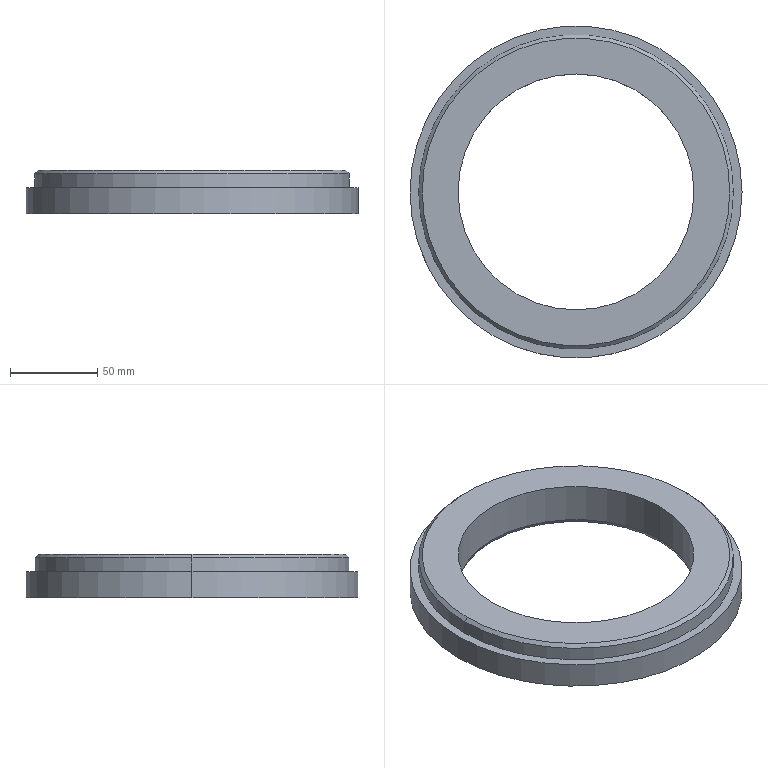Part | SolidWorks | features Chamfer 2, 3DProfileFeature 1, Extrusion 1, HoleWzd 1, ICE 1 | 1 solid | 37 faces | box 190 x 190 x 25 mm | volume 309604 mm3 | cylinder 18 | cone 16 | plane 3 | commonest cylinder face diameters 10.5 x12 135 x2 180 x2 190 x2
STEP:
#1=CARTESIAN_POINT('',(45.5,69.715,20.));
#2=VERTEX_POINT('',#1);
#3=CARTESIAN_POINT('',(35.,69.715,20.));
#4=VERTEX_POINT('',#3);
#5=CARTESIAN_POINT('',(40.25,69.715,20.));
#6=DIRECTION('',(0.,0.,-1.));
#7=DIRECTION('',(-1.,0.,0.));
#8=AXIS2_PLACEMENT_3D('',#5,#6,#7);
#9=CIRCLE('',#8,5.25);
#10=EDGE_CURVE('',#2,#4,#9,.T.);
#11=ORIENTED_EDGE('',*,*,#10,.F.);
#12=CARTESIAN_POINT('',(45.5,69.715,0.));
#13=VERTEX_POINT('',#12);
#14=CARTESIAN_POINT('',(45.5,69.715,0.));
#15=DIRECTION('',(0.,0.,-1.));
#16=VECTOR('',#15,1000.);
#17=LINE('',#14,#16);
#18=EDGE_CURVE('',#2,#13,#17,.T.);
#19=ORIENTED_EDGE('',*,*,#18,.T.);
#20=CARTESIAN_POINT('',(35.,69.715,0.));
#21=VERTEX_POINT('',#20);
#22=CARTESIAN_POINT('',(40.25,69.715,0.));
#23=DIRECTION('',(0.,0.,-1.));
#24=DIRECTION('',(-1.,0.,0.));
#25=AXIS2_PLACEMENT_3D('',#22,#23,#24);
#26=CIRCLE('',#25,5.25);
#27=EDGE_CURVE('',#13,#21,#26,.T.);
#28=ORIENTED_EDGE('',*,*,#27,.T.);
#29=CARTESIAN_POINT('',(35.,69.715,0.));
#30=DIRECTION('',(0.,0.,-1.));
#31=VECTOR('',#30,1000.);
#32=LINE('',#29,#31);
#33=EDGE_CURVE('',#4,#21,#32,.T.);
#34=ORIENTED_EDGE('',*,*,#33,.F.);
#35=EDGE_LOOP('',(#11,#19,#28,#34));
#36=FACE_OUTER_BOUND('',#35,.T.);
#37=CARTESIAN_POINT('',(40.25,69.715,0.));
#38=DIRECTION('',(0.,0.,-1.));
#39=DIRECTION('',(-1.,0.,0.));
#40=AXIS2_PLACEMENT_3D('',#37,#38,#39);
#41=CYLINDRICAL_SURFACE('',#40,5.25);
#42=ADVANCED_FACE('',(#36),#41,.F.);
#43=CARTESIAN_POINT('',(40.25,69.715,23.155));
#44=VERTEX_POINT('',#43);
#45=CARTESIAN_POINT('',(35.,69.715,20.));
#46=DIRECTION('',(-0.8572,0.,-0.515));
#47=VECTOR('',#46,1000.);
#48=LINE('',#45,#47);
#49=EDGE_CURVE('',#44,#4,#48,.T.);
#50=ORIENTED_EDGE('',*,*,#49,.F.);
#51=CARTESIAN_POINT('',(45.5,69.715,20.));
#52=DIRECTION('',(0.8572,0.,-0.515));
#53=VECTOR('',#52,1000.);
#54=LINE('',#51,#53);
#55=EDGE_CURVE('',#44,#2,#54,.T.);
#56=ORIENTED_EDGE('',*,*,#55,.T.);
#57=ORIENTED_EDGE('',*,*,#10,.T.);
#58=EDGE_LOOP('',(#50,#56,#57));
#59=FACE_OUTER_BOUND('',#58,.T.);
#60=CARTESIAN_POINT('',(40.25,69.715,20.));
#61=DIRECTION('',(0.,0.,-1.));
#62=DIRECTION('',(-1.,0.,0.));
#63=AXIS2_PLACEMENT_3D('',#60,#61,#62);
#64=CONICAL_SURFACE('',#63,5.25,1.03);
#65=ADVANCED_FACE('',(#59),#64,.F.);
#66=CARTESIAN_POINT('',(-35.,69.715,20.));
#67=VERTEX_POINT('',#66);
#68=CARTESIAN_POINT('',(-45.5,69.715,20.));
#69=VERTEX_POINT('',#68);
#70=CARTESIAN_POINT('',(-40.25,69.715,20.));
#71=DIRECTION('',(0.,0.,-1.));
#72=DIRECTION('',(-1.,0.,0.));
#73=AXIS2_PLACEMENT_3D('',#70,#71,#72);
#74=CIRCLE('',#73,5.25);
#75=EDGE_CURVE('',#67,#69,#74,.T.);
#76=ORIENTED_EDGE('',*,*,#75,.F.);
#77=CARTESIAN_POINT('',(-35.,69.715,0.));
#78=VERTEX_POINT('',#77);
#79=CARTESIAN_POINT('',(-35.,69.715,0.));
#80=DIRECTION('',(0.,0.,-1.));
#81=VECTOR('',#80,1000.);
#82=LINE('',#79,#81);
#83=EDGE_CURVE('',#67,#78,#82,.T.);
#84=ORIENTED_EDGE('',*,*,#83,.T.);
#85=CARTESIAN_POINT('',(-45.5,69.715,0.));
#86=VERTEX_POINT('',#85);
#87=CARTESIAN_POINT('',(-40.25,69.715,0.));
#88=DIRECTION('',(0.,0.,-1.));
#89=DIRECTION('',(-1.,0.,0.));
#90=AXIS2_PLACEMENT_3D('',#87,#88,#89);
#91=CIRCLE('',#90,5.25);
#92=EDGE_CURVE('',#78,#86,#91,.T.);
#93=ORIENTED_EDGE('',*,*,#92,.T.);
#94=CARTESIAN_POINT('',(-45.5,69.715,0.));
#95=DIRECTION('',(0.,0.,-1.));
#96=VECTOR('',#95,1000.);
#97=LINE('',#94,#96);
#98=EDGE_CURVE('',#69,#86,#97,.T.);
#99=ORIENTED_EDGE('',*,*,#98,.F.);
#100=EDGE_LOOP('',(#76,#84,#93,#99));
#101=FACE_OUTER_BOUND('',#100,.T.);
#102=CARTESIAN_POINT('',(-40.25,69.715,0.));
#103=DIRECTION('',(0.,0.,-1.));
#104=DIRECTION('',(-1.,0.,0.));
#105=AXIS2_PLACEMENT_3D('',#102,#103,#104);
#106=CYLINDRICAL_SURFACE('',#105,5.25);
#107=ADVANCED_FACE('',(#101),#106,.F.);
#108=CARTESIAN_POINT('',(-40.25,69.715,23.155));
#109=VERTEX_POINT('',#108);
#110=CARTESIAN_POINT('',(-45.5,69.715,20.));
#111=DIRECTION('',(-0.8572,0.,-0.515));
#112=VECTOR('',#111,1000.);
#113=LINE('',#110,#112);
#114=EDGE_CURVE('',#109,#69,#113,.T.);
#115=ORIENTED_EDGE('',*,*,#114,.F.);
#116=CARTESIAN_POINT('',(-35.,69.715,20.));
#117=DIRECTION('',(0.8572,0.,-0.515));
#118=VECTOR('',#117,1000.);
#119=LINE('',#116,#118);
#120=EDGE_CURVE('',#109,#67,#119,.T.);
#121=ORIENTED_EDGE('',*,*,#120,.T.);
#122=ORIENTED_EDGE('',*,*,#75,.T.);
#123=EDGE_LOOP('',(#115,#121,#122));
#124=FACE_OUTER_BOUND('',#123,.T.);
#125=CARTESIAN_POINT('',(-40.25,69.715,20.));
#126=DIRECTION('',(0.,0.,-1.));
#127=DIRECTION('',(-1.,0.,0.));
#128=AXIS2_PLACEMENT_3D('',#125,#126,#127);
#129=CONICAL_SURFACE('',#128,5.25,1.03);
#130=ADVANCED_FACE('',(#124),#129,.F.);
#131=CARTESIAN_POINT('',(-75.25,0.,20.));
#132=VERTEX_POINT('',#131);
#133=CARTESIAN_POINT('',(-85.75,0.,20.));
#134=VERTEX_POINT('',#133);
#135=CARTESIAN_POINT('',(-80.5,0.,20.));
#136=DIRECTION('',(0.,0.,-1.));
#137=DIRECTION('',(-1.,0.,0.));
#138=AXIS2_PLACEMENT_3D('',#135,#136,#137);
#139=CIRCLE('',#138,5.25);
#140=EDGE_CURVE('',#132,#134,#139,.T.);
#141=ORIENTED_EDGE('',*,*,#140,.F.);
#142=CARTESIAN_POINT('',(-75.25,0.,0.));
#143=VERTEX_POINT('',#142);
#144=CARTESIAN_POINT('',(-75.25,0.,0.));
#145=DIRECTION('',(0.,0.,-1.));
#146=VECTOR('',#145,1000.);
#147=LINE('',#144,#146);
#148=EDGE_CURVE('',#132,#143,#147,.T.);
#149=ORIENTED_EDGE('',*,*,#148,.T.);
#150=CARTESIAN_POINT('',(-85.75,0.,0.));
#151=VERTEX_POINT('',#150);
#152=CARTESIAN_POINT('',(-80.5,0.,0.));
#153=DIRECTION('',(0.,0.,-1.));
#154=DIRECTION('',(-1.,0.,0.));
#155=AXIS2_PLACEMENT_3D('',#152,#153,#154);
#156=CIRCLE('',#155,5.25);
#157=EDGE_CURVE('',#143,#151,#156,.T.);
#158=ORIENTED_EDGE('',*,*,#157,.T.);
#159=CARTESIAN_POINT('',(-85.75,0.,0.));
#160=DIRECTION('',(0.,0.,-1.));
#161=VECTOR('',#160,1000.);
#162=LINE('',#159,#161);
#163=EDGE_CURVE('',#134,#151,#162,.T.);
#164=ORIENTED_EDGE('',*,*,#163,.F.);
#165=EDGE_LOOP('',(#141,#149,#158,#164));
#166=FACE_OUTER_BOUND('',#165,.T.);
#167=CARTESIAN_POINT('',(-80.5,0.,0.));
#168=DIRECTION('',(0.,0.,-1.));
#169=DIRECTION('',(-1.,0.,0.));
#170=AXIS2_PLACEMENT_3D('',#167,#168,#169);
#171=CYLINDRICAL_SURFACE('',#170,5.25);
#172=ADVANCED_FACE('',(#166),#171,.F.);
#173=CARTESIAN_POINT('',(-80.5,0.,23.155));
#174=VERTEX_POINT('',#173);
#175=CARTESIAN_POINT('',(-85.75,0.,20.));
#176=DIRECTION('',(-0.8572,0.,-0.515));
#177=VECTOR('',#176,1000.);
#178=LINE('',#175,#177);
#179=EDGE_CURVE('',#174,#134,#178,.T.);
#180=ORIENTED_EDGE('',*,*,#179,.F.);
#181=CARTESIAN_POINT('',(-75.25,0.,20.));
#182=DIRECTION('',(0.8572,0.,-0.515));
#183=VECTOR('',#182,1000.);
#184=LINE('',#181,#183);
#185=EDGE_CURVE('',#174,#132,#184,.T.);
#186=ORIENTED_EDGE('',*,*,#185,.T.);
#187=ORIENTED_EDGE('',*,*,#140,.T.);
#188=EDGE_LOOP('',(#180,#186,#187));
#189=FACE_OUTER_BOUND('',#188,.T.);
#190=CARTESIAN_POINT('',(-80.5,0.,20.));
#191=DIRECTION('',(0.,0.,-1.));
#192=DIRECTION('',(-1.,0.,0.));
#193=AXIS2_PLACEMENT_3D('',#190,#191,#192);
#194=CONICAL_SURFACE('',#193,5.25,1.03);
#195=ADVANCED_FACE('',(#189),#194,.F.);
#196=CARTESIAN_POINT('',(-35.,-69.715,20.));
#197=VERTEX_POINT('',#196);
#198=CARTESIAN_POINT('',(-45.5,-69.715,20.));
#199=VERTEX_POINT('',#198);
#200=CARTESIAN_POINT('',(-40.25,-69.715,20.));
#201=DIRECTION('',(0.,0.,-1.));
#202=DIRECTION('',(-1.,0.,0.));
#203=AXIS2_PLACEMENT_3D('',#200,#201,#202);
#204=CIRCLE('',#203,5.25);
#205=EDGE_CURVE('',#197,#199,#204,.T.);
#206=ORIENTED_EDGE('',*,*,#205,.F.);
#207=CARTESIAN_POINT('',(-35.,-69.715,0.));
#208=VERTEX_POINT('',#207);
#209=CARTESIAN_POINT('',(-35.,-69.715,0.));
#210=DIRECTION('',(0.,0.,-1.));
#211=VECTOR('',#210,1000.);
#212=LINE('',#209,#211);
#213=EDGE_CURVE('',#197,#208,#212,.T.);
#214=ORIENTED_EDGE('',*,*,#213,.T.);
#215=CARTESIAN_POINT('',(-45.5,-69.715,0.));
#216=VERTEX_POINT('',#215);
#217=CARTESIAN_POINT('',(-40.25,-69.715,0.));
#218=DIRECTION('',(0.,0.,-1.));
#219=DIRECTION('',(-1.,0.,0.));
#220=AXIS2_PLACEMENT_3D('',#217,#218,#219);
#221=CIRCLE('',#220,5.25);
#222=EDGE_CURVE('',#208,#216,#221,.T.);
#223=ORIENTED_EDGE('',*,*,#222,.T.);
#224=CARTESIAN_POINT('',(-45.5,-69.715,0.));
#225=DIRECTION('',(0.,0.,-1.));
#226=VECTOR('',#225,1000.);
#227=LINE('',#224,#226);
#228=EDGE_CURVE('',#199,#216,#227,.T.);
#229=ORIENTED_EDGE('',*,*,#228,.F.);
#230=EDGE_LOOP('',(#206,#214,#223,#229));
#231=FACE_OUTER_BOUND('',#230,.T.);
#232=CARTESIAN_POINT('',(-40.25,-69.715,0.));
#233=DIRECTION('',(0.,0.,-1.));
#234=DIRECTION('',(-1.,0.,0.));
#235=AXIS2_PLACEMENT_3D('',#232,#233,#234);
#236=CYLINDRICAL_SURFACE('',#235,5.25);
#237=ADVANCED_FACE('',(#231),#236,.F.);
#238=CARTESIAN_POINT('',(-40.25,-69.715,23.155));
#239=VERTEX_POINT('',#238);
#240=CARTESIAN_POINT('',(-45.5,-69.715,20.));
#241=DIRECTION('',(-0.8572,0.,-0.515));
#242=VECTOR('',#241,1000.);
#243=LINE('',#240,#242);
#244=EDGE_CURVE('',#239,#199,#243,.T.);
#245=ORIENTED_EDGE('',*,*,#244,.F.);
#246=CARTESIAN_POINT('',(-35.,-69.715,20.));
#247=DIRECTION('',(0.8572,0.,-0.515));
#248=VECTOR('',#247,1000.);
#249=LINE('',#246,#248);
#250=EDGE_CURVE('',#239,#197,#249,.T.);
#251=ORIENTED_EDGE('',*,*,#250,.T.);
#252=ORIENTED_EDGE('',*,*,#205,.T.);
#253=EDGE_LOOP('',(#245,#251,#252));
#254=FACE_OUTER_BOUND('',#253,.T.);
#255=CARTESIAN_POINT('',(-40.25,-69.715,20.));
#256=DIRECTION('',(0.,0.,-1.));
#257=DIRECTION('',(-1.,0.,0.));
#258=AXIS2_PLACEMENT_3D('',#255,#256,#257);
#259=CONICAL_SURFACE('',#258,5.25,1.03);
#260=ADVANCED_FACE('',(#254),#259,.F.);
#261=CARTESIAN_POINT('',(85.75,0.,20.));
#262=VERTEX_POINT('',#261);
#263=CARTESIAN_POINT('',(75.25,0.,20.));
#264=VERTEX_POINT('',#263);
#265=CARTESIAN_POINT('',(80.5,0.,20.));
#266=DIRECTION('',(0.,0.,-1.));
#267=DIRECTION('',(-1.,0.,0.));
#268=AXIS2_PLACEMENT_3D('',#265,#266,#267);
#269=CIRCLE('',#268,5.25);
#270=EDGE_CURVE('',#262,#264,#269,.T.);
#271=ORIENTED_EDGE('',*,*,#270,.F.);
#272=CARTESIAN_POINT('',(85.75,0.,0.));
#273=VERTEX_POINT('',#272);
#274=CARTESIAN_POINT('',(85.75,0.,0.));
#275=DIRECTION('',(0.,0.,-1.));
#276=VECTOR('',#275,1000.);
#277=LINE('',#274,#276);
#278=EDGE_CURVE('',#262,#273,#277,.T.);
#279=ORIENTED_EDGE('',*,*,#278,.T.);
#280=CARTESIAN_POINT('',(75.25,0.,0.));
#281=VERTEX_POINT('',#280);
#282=CARTESIAN_POINT('',(80.5,0.,0.));
#283=DIRECTION('',(0.,0.,-1.));
#284=DIRECTION('',(-1.,0.,0.));
#285=AXIS2_PLACEMENT_3D('',#282,#283,#284);
#286=CIRCLE('',#285,5.25);
#287=EDGE_CURVE('',#273,#281,#286,.T.);
#288=ORIENTED_EDGE('',*,*,#287,.T.);
#289=CARTESIAN_POINT('',(75.25,0.,0.));
#290=DIRECTION('',(0.,0.,-1.));
#291=VECTOR('',#290,1000.);
#292=LINE('',#289,#291);
#293=EDGE_CURVE('',#264,#281,#292,.T.);
#294=ORIENTED_EDGE('',*,*,#293,.F.);
#295=EDGE_LOOP('',(#271,#279,#288,#294));
#296=FACE_OUTER_BOUND('',#295,.T.);
#297=CARTESIAN_POINT('',(80.5,0.,0.));
#298=DIRECTION('',(0.,0.,-1.));
#299=DIRECTION('',(-1.,0.,0.));
#300=AXIS2_PLACEMENT_3D('',#297,#298,#299);
#301=CYLINDRICAL_SURFACE('',#300,5.25);
#302=ADVANCED_FACE('',(#296),#301,.F.);
#303=CARTESIAN_POINT('',(80.5,0.,23.155));
#304=VERTEX_POINT('',#303);
#305=CARTESIAN_POINT('',(75.25,0.,20.));
#306=DIRECTION('',(-0.8572,0.,-0.515));
#307=VECTOR('',#306,1000.);
#308=LINE('',#305,#307);
#309=EDGE_CURVE('',#304,#264,#308,.T.);
#310=ORIENTED_EDGE('',*,*,#309,.F.);
#311=CARTESIAN_POINT('',(85.75,0.,20.));
#312=DIRECTION('',(0.8572,0.,-0.515));
#313=VECTOR('',#312,1000.);
#314=LINE('',#311,#313);
#315=EDGE_CURVE('',#304,#262,#314,.T.);
#316=ORIENTED_EDGE('',*,*,#315,.T.);
#317=ORIENTED_EDGE('',*,*,#270,.T.);
#318=EDGE_LOOP('',(#310,#316,#317));
#319=FACE_OUTER_BOUND('',#318,.T.);
#320=CARTESIAN_POINT('',(80.5,0.,20.));
#321=DIRECTION('',(0.,0.,-1.));
#322=DIRECTION('',(-1.,0.,0.));
#323=AXIS2_PLACEMENT_3D('',#320,#321,#322);
#324=CONICAL_SURFACE('',#323,5.25,1.03);
#325=ADVANCED_FACE('',(#319),#324,.F.);
#326=CARTESIAN_POINT('',(45.5,-69.715,20.));
#327=VERTEX_POINT('',#326);
#328=CARTESIAN_POINT('',(35.,-69.715,20.));
#329=VERTEX_POINT('',#328);
#330=CARTESIAN_POINT('',(40.25,-69.715,20.));
#331=DIRECTION('',(0.,0.,-1.));
#332=DIRECTION('',(-1.,0.,0.));
#333=AXIS2_PLACEMENT_3D('',#330,#331,#332);
#334=CIRCLE('',#333,5.25);
#335=EDGE_CURVE('',#327,#329,#334,.T.);
#336=ORIENTED_EDGE('',*,*,#335,.F.);
#337=CARTESIAN_POINT('',(45.5,-69.715,0.));
#338=VERTEX_POINT('',#337);
#339=CARTESIAN_POINT('',(45.5,-69.715,0.));
#340=DIRECTION('',(0.,0.,-1.));
#341=VECTOR('',#340,1000.);
#342=LINE('',#339,#341);
#343=EDGE_CURVE('',#327,#338,#342,.T.);
#344=ORIENTED_EDGE('',*,*,#343,.T.);
#345=CARTESIAN_POINT('',(35.,-69.715,0.));
#346=VERTEX_POINT('',#345);
#347=CARTESIAN_POINT('',(40.25,-69.715,0.));
#348=DIRECTION('',(0.,0.,-1.));
#349=DIRECTION('',(-1.,0.,0.));
#350=AXIS2_PLACEMENT_3D('',#347,#348,#349);
#351=CIRCLE('',#350,5.25);
#352=EDGE_CURVE('',#338,#346,#351,.T.);
#353=ORIENTED_EDGE('',*,*,#352,.T.);
#354=CARTESIAN_POINT('',(35.,-69.715,0.));
#355=DIRECTION('',(0.,0.,-1.));
#356=VECTOR('',#355,1000.);
#357=LINE('',#354,#356);
#358=EDGE_CURVE('',#329,#346,#357,.T.);
#359=ORIENTED_EDGE('',*,*,#358,.F.);
#360=EDGE_LOOP('',(#336,#344,#353,#359));
#361=FACE_OUTER_BOUND('',#360,.T.);
#362=CARTESIAN_POINT('',(40.25,-69.715,0.));
#363=DIRECTION('',(0.,0.,-1.));
#364=DIRECTION('',(-1.,0.,0.));
#365=AXIS2_PLACEMENT_3D('',#362,#363,#364);
#366=CYLINDRICAL_SURFACE('',#365,5.25);
#367=ADVANCED_FACE('',(#361),#366,.F.);
#368=CARTESIAN_POINT('',(40.25,-69.715,23.155));
#369=VERTEX_POINT('',#368);
#370=CARTESIAN_POINT('',(35.,-69.715,20.));
#371=DIRECTION('',(-0.8572,0.,-0.515));
#372=VECTOR('',#371,1000.);
#373=LINE('',#370,#372);
#374=EDGE_CURVE('',#369,#329,#373,.T.);
#375=ORIENTED_EDGE('',*,*,#374,.F.);
#376=CARTESIAN_POINT('',(45.5,-69.715,20.));
#377=DIRECTION('',(0.8572,0.,-0.515));
#378=VECTOR('',#377,1000.);
#379=LINE('',#376,#378);
#380=EDGE_CURVE('',#369,#327,#379,.T.);
#381=ORIENTED_EDGE('',*,*,#380,.T.);
#382=ORIENTED_EDGE('',*,*,#335,.T.);
#383=EDGE_LOOP('',(#375,#381,#382));
#384=FACE_OUTER_BOUND('',#383,.T.);
#385=CARTESIAN_POINT('',(40.25,-69.715,20.));
#386=DIRECTION('',(0.,0.,-1.));
#387=DIRECTION('',(-1.,0.,0.));
#388=AXIS2_PLACEMENT_3D('',#385,#386,#387);
#389=CONICAL_SURFACE('',#388,5.25,1.03);
#390=ADVANCED_FACE('',(#384),#389,.F.);
#391=CARTESIAN_POINT('',(67.5,0.,1.8));
#392=VERTEX_POINT('',#391);
#393=CARTESIAN_POINT('',(-67.5,0.,1.8));
#394=VERTEX_POINT('',#393);
#395=CARTESIAN_POINT('',(0.,0.,1.8));
#396=DIRECTION('',(0.,0.,-1.));
#397=DIRECTION('',(1.,0.,0.));
#398=AXIS2_PLACEMENT_3D('',#395,#396,#397);
#399=CIRCLE('',#398,67.5);
#400=EDGE_CURVE('',#392,#394,#399,.T.);
#401=ORIENTED_EDGE('',*,*,#400,.F.);
#402=CARTESIAN_POINT('',(68.155,0.,0.));
#403=VERTEX_POINT('',#402);
#404=CARTESIAN_POINT('',(68.155,0.,0.));
#405=DIRECTION('',(0.342,0.,-0.9397));
#406=VECTOR('',#405,1000.);
#407=LINE('',#404,#406);
#408=EDGE_CURVE('',#392,#403,#407,.T.);
#409=ORIENTED_EDGE('',*,*,#408,.T.);
#410=CARTESIAN_POINT('',(-68.155,0.,0.));
#411=VERTEX_POINT('',#410);
#412=CARTESIAN_POINT('',(0.,0.,0.));
#413=DIRECTION('',(0.,0.,1.));
#414=DIRECTION('',(1.,0.,0.));
#415=AXIS2_PLACEMENT_3D('',#412,#413,#414);
#416=CIRCLE('',#415,68.155);
#417=EDGE_CURVE('',#411,#403,#416,.T.);
#418=ORIENTED_EDGE('',*,*,#417,.F.);
#419=CARTESIAN_POINT('',(-68.155,0.,0.));
#420=DIRECTION('',(-0.342,0.,-0.9397));
#421=VECTOR('',#420,1000.);
#422=LINE('',#419,#421);
#423=EDGE_CURVE('',#394,#411,#422,.T.);
#424=ORIENTED_EDGE('',*,*,#423,.F.);
#425=EDGE_LOOP('',(#401,#409,#418,#424));
#426=FACE_OUTER_BOUND('',#425,.T.);
#427=CARTESIAN_POINT('',(0.,0.,0.));
#428=DIRECTION('',(0.,0.,-1.));
#429=DIRECTION('',(-1.,0.,0.));
#430=AXIS2_PLACEMENT_3D('',#427,#428,#429);
#431=CONICAL_SURFACE('',#430,68.155,0.3491);
#432=ADVANCED_FACE('',(#426),#431,.F.);
#433=CARTESIAN_POINT('',(88.,0.,25.));
#434=VERTEX_POINT('',#433);
#435=CARTESIAN_POINT('',(-88.,0.,25.));
#436=VERTEX_POINT('',#435);
#437=CARTESIAN_POINT('',(0.,0.,25.));
#438=DIRECTION('',(0.,0.,1.));
#439=DIRECTION('',(1.,0.,0.));
#440=AXIS2_PLACEMENT_3D('',#437,#438,#439);
#441=CIRCLE('',#440,88.);
#442=EDGE_CURVE('',#434,#436,#441,.T.);
#443=ORIENTED_EDGE('',*,*,#442,.F.);
#444=CARTESIAN_POINT('',(90.,0.,23.));
#445=VERTEX_POINT('',#444);
#446=CARTESIAN_POINT('',(88.,0.,25.));
#447=DIRECTION('',(0.7071,0.,-0.7071));
#448=VECTOR('',#447,1000.);
#449=LINE('',#446,#448);
#450=EDGE_CURVE('',#434,#445,#449,.T.);
#451=ORIENTED_EDGE('',*,*,#450,.T.);
#452=CARTESIAN_POINT('',(-90.,0.,23.));
#453=VERTEX_POINT('',#452);
#454=CARTESIAN_POINT('',(0.,0.,23.));
#455=DIRECTION('',(0.,0.,-1.));
#456=DIRECTION('',(1.,0.,0.));
#457=AXIS2_PLACEMENT_3D('',#454,#455,#456);
#458=CIRCLE('',#457,90.);
#459=EDGE_CURVE('',#453,#445,#458,.T.);
#460=ORIENTED_EDGE('',*,*,#459,.F.);
#461=CARTESIAN_POINT('',(-88.,0.,25.));
#462=DIRECTION('',(-0.7071,0.,-0.7071));
#463=VECTOR('',#462,1000.);
#464=LINE('',#461,#463);
#465=EDGE_CURVE('',#436,#453,#464,.T.);
#466=ORIENTED_EDGE('',*,*,#465,.F.);
#467=EDGE_LOOP('',(#443,#451,#460,#466));
#468=FACE_OUTER_BOUND('',#467,.T.);
#469=CARTESIAN_POINT('',(0.,0.,25.));
#470=DIRECTION('',(0.,0.,-1.));
#471=DIRECTION('',(-1.,0.,0.));
#472=AXIS2_PLACEMENT_3D('',#469,#470,#471);
#473=CONICAL_SURFACE('',#472,88.,0.7854);
#474=ADVANCED_FACE('',(#468),#473,.T.);
#475=ORIENTED_EDGE('',*,*,#459,.T.);
#476=CARTESIAN_POINT('',(90.,0.,15.));
#477=VERTEX_POINT('',#476);
#478=CARTESIAN_POINT('',(90.,0.,25.));
#479=DIRECTION('',(0.,0.,-1.));
#480=VECTOR('',#479,1000.);
#481=LINE('',#478,#480);
#482=EDGE_CURVE('',#445,#477,#481,.T.);
#483=ORIENTED_EDGE('',*,*,#482,.T.);
#484=CARTESIAN_POINT('',(-90.,0.,15.));
#485=VERTEX_POINT('',#484);
#486=CARTESIAN_POINT('',(0.,0.,15.));
#487=DIRECTION('',(0.,0.,1.));
#488=DIRECTION('',(1.,0.,0.));
#489=AXIS2_PLACEMENT_3D('',#486,#487,#488);
#490=CIRCLE('',#489,90.);
#491=EDGE_CURVE('',#477,#485,#490,.T.);
#492=ORIENTED_EDGE('',*,*,#491,.T.);
#493=CARTESIAN_POINT('',(-90.,0.,25.));
#494=DIRECTION('',(0.,0.,-1.));
#495=VECTOR('',#494,1000.);
#496=LINE('',#493,#495);
#497=EDGE_CURVE('',#453,#485,#496,.T.);
#498=ORIENTED_EDGE('',*,*,#497,.F.);
#499=EDGE_LOOP('',(#475,#483,#492,#498));
#500=FACE_OUTER_BOUND('',#499,.T.);
#501=CARTESIAN_POINT('',(0.,0.,25.));
#502=DIRECTION('',(0.,0.,-1.));
#503=DIRECTION('',(-1.,0.,0.));
#504=AXIS2_PLACEMENT_3D('',#501,#502,#503);
#505=CYLINDRICAL_SURFACE('',#504,90.);
#506=ADVANCED_FACE('',(#500),#505,.T.);
#507=CARTESIAN_POINT('',(-67.5,0.,25.));
#508=VERTEX_POINT('',#507);
#509=CARTESIAN_POINT('',(67.5,0.,25.));
#510=VERTEX_POINT('',#509);
#511=CARTESIAN_POINT('',(0.,0.,25.));
#512=DIRECTION('',(0.,0.,1.));
#513=DIRECTION('',(1.,0.,0.));
#514=AXIS2_PLACEMENT_3D('',#511,#512,#513);
#515=CIRCLE('',#514,67.5);
#516=EDGE_CURVE('',#508,#510,#515,.T.);
#517=ORIENTED_EDGE('',*,*,#516,.T.);
#518=CARTESIAN_POINT('',(67.5,0.,15.));
#519=DIRECTION('',(0.,0.,-1.));
#520=VECTOR('',#519,1000.);
#521=LINE('',#518,#520);
#522=EDGE_CURVE('',#510,#392,#521,.T.);
#523=ORIENTED_EDGE('',*,*,#522,.T.);
#524=ORIENTED_EDGE('',*,*,#400,.T.);
#525=CARTESIAN_POINT('',(-67.5,0.,15.));
#526=DIRECTION('',(0.,0.,-1.));
#527=VECTOR('',#526,1000.);
#528=LINE('',#525,#527);
#529=EDGE_CURVE('',#508,#394,#528,.T.);
#530=ORIENTED_EDGE('',*,*,#529,.F.);
#531=EDGE_LOOP('',(#517,#523,#524,#530));
#532=FACE_OUTER_BOUND('',#531,.T.);
#533=CARTESIAN_POINT('',(0.,0.,15.));
#534=DIRECTION('',(0.,0.,-1.));
#535=DIRECTION('',(-1.,0.,0.));
#536=AXIS2_PLACEMENT_3D('',#533,#534,#535);
#537=CYLINDRICAL_SURFACE('',#536,67.5);
#538=ADVANCED_FACE('',(#532),#537,.F.);
#539=CARTESIAN_POINT('',(95.,0.,15.));
#540=VERTEX_POINT('',#539);
#541=CARTESIAN_POINT('',(-95.,0.,15.));
#542=VERTEX_POINT('',#541);
#543=CARTESIAN_POINT('',(0.,0.,15.));
#544=DIRECTION('',(0.,0.,1.));
#545=DIRECTION('',(1.,0.,0.));
#546=AXIS2_PLACEMENT_3D('',#543,#544,#545);
#547=CIRCLE('',#546,95.);
#548=EDGE_CURVE('',#540,#542,#547,.T.);
#549=ORIENTED_EDGE('',*,*,#548,.F.);
#550=CARTESIAN_POINT('',(95.,0.,0.));
#551=VERTEX_POINT('',#550);
#552=CARTESIAN_POINT('',(95.,0.,15.));
#553=DIRECTION('',(0.,0.,-1.));
#554=VECTOR('',#553,1000.);
#555=LINE('',#552,#554);
#556=EDGE_CURVE('',#540,#551,#555,.T.);
#557=ORIENTED_EDGE('',*,*,#556,.T.);
#558=CARTESIAN_POINT('',(-95.,0.,0.));
#559=VERTEX_POINT('',#558);
#560=CARTESIAN_POINT('',(0.,0.,0.));
#561=DIRECTION('',(0.,0.,1.));
#562=DIRECTION('',(1.,0.,0.));
#563=AXIS2_PLACEMENT_3D('',#560,#561,#562);
#564=CIRCLE('',#563,95.);
#565=EDGE_CURVE('',#551,#559,#564,.T.);
#566=ORIENTED_EDGE('',*,*,#565,.T.);
#567=CARTESIAN_POINT('',(-95.,0.,15.));
#568=DIRECTION('',(0.,0.,-1.));
#569=VECTOR('',#568,1000.);
#570=LINE('',#567,#569);
#571=EDGE_CURVE('',#542,#559,#570,.T.);
#572=ORIENTED_EDGE('',*,*,#571,.F.);
#573=EDGE_LOOP('',(#549,#557,#566,#572));
#574=FACE_OUTER_BOUND('',#573,.T.);
#575=CARTESIAN_POINT('',(0.,0.,15.));
#576=DIRECTION('',(0.,0.,-1.));
#577=DIRECTION('',(-1.,0.,0.));
#578=AXIS2_PLACEMENT_3D('',#575,#576,#577);
#579=CYLINDRICAL_SURFACE('',#578,95.);
#580=ADVANCED_FACE('',(#574),#579,.T.);
#581=CARTESIAN_POINT('',(0.,0.,15.));
#582=DIRECTION('',(0.,0.,1.));
#583=DIRECTION('',(1.,0.,0.));
#584=AXIS2_PLACEMENT_3D('',#581,#582,#583);
#585=CIRCLE('',#584,95.);
#586=EDGE_CURVE('',#542,#540,#585,.T.);
#587=ORIENTED_EDGE('',*,*,#586,.T.);
#588=ORIENTED_EDGE('',*,*,#548,.T.);
#589=EDGE_LOOP('',(#587,#588));
#590=FACE_OUTER_BOUND('',#589,.T.);
#591=CARTESIAN_POINT('',(0.,0.,15.));
#592=DIRECTION('',(0.,0.,1.));
#593=DIRECTION('',(1.,0.,0.));
#594=AXIS2_PLACEMENT_3D('',#591,#592,#593);
#595=CIRCLE('',#594,90.);
#596=EDGE_CURVE('',#485,#477,#595,.T.);
#597=ORIENTED_EDGE('',*,*,#596,.F.);
#598=ORIENTED_EDGE('',*,*,#491,.F.);
#599=EDGE_LOOP('',(#597,#598));
#600=FACE_BOUND('',#599,.T.);
#601=CARTESIAN_POINT('',(0.,0.,15.));
#602=DIRECTION('',(0.,0.,1.));
#603=DIRECTION('',(1.,0.,0.));
#604=AXIS2_PLACEMENT_3D('',#601,#602,#603);
#605=PLANE('',#604);
#606=ADVANCED_FACE('',(#590,#600),#605,.T.);
#607=CARTESIAN_POINT('',(40.25,69.715,0.));
#608=DIRECTION('',(0.,0.,-1.));
#609=DIRECTION('',(-1.,0.,0.));
#610=AXIS2_PLACEMENT_3D('',#607,#608,#609);
#611=CIRCLE('',#610,5.25);
#612=EDGE_CURVE('',#21,#13,#611,.T.);
#613=ORIENTED_EDGE('',*,*,#612,.F.);
#614=ORIENTED_EDGE('',*,*,#27,.F.);
#615=EDGE_LOOP('',(#613,#614));
#616=FACE_BOUND('',#615,.T.);
#617=CARTESIAN_POINT('',(-40.25,69.715,0.));
#618=DIRECTION('',(0.,0.,-1.));
#619=DIRECTION('',(-1.,0.,0.));
#620=AXIS2_PLACEMENT_3D('',#617,#618,#619);
#621=CIRCLE('',#620,5.25);
#622=EDGE_CURVE('',#86,#78,#621,.T.);
#623=ORIENTED_EDGE('',*,*,#622,.F.);
#624=ORIENTED_EDGE('',*,*,#92,.F.);
#625=EDGE_LOOP('',(#623,#624));
#626=FACE_BOUND('',#625,.T.);
#627=CARTESIAN_POINT('',(-80.5,0.,0.));
#628=DIRECTION('',(0.,0.,-1.));
#629=DIRECTION('',(-1.,0.,0.));
#630=AXIS2_PLACEMENT_3D('',#627,#628,#629);
#631=CIRCLE('',#630,5.25);
#632=EDGE_CURVE('',#151,#143,#631,.T.);
#633=ORIENTED_EDGE('',*,*,#632,.F.);
#634=ORIENTED_EDGE('',*,*,#157,.F.);
#635=EDGE_LOOP('',(#633,#634));
#636=FACE_BOUND('',#635,.T.);
#637=CARTESIAN_POINT('',(-40.25,-69.715,0.));
#638=DIRECTION('',(0.,0.,-1.));
#639=DIRECTION('',(-1.,0.,0.));
#640=AXIS2_PLACEMENT_3D('',#637,#638,#639);
#641=CIRCLE('',#640,5.25);
#642=EDGE_CURVE('',#216,#208,#641,.T.);
#643=ORIENTED_EDGE('',*,*,#642,.F.);
#644=ORIENTED_EDGE('',*,*,#222,.F.);
#645=EDGE_LOOP('',(#643,#644));
#646=FACE_BOUND('',#645,.T.);
#647=CARTESIAN_POINT('',(80.5,0.,0.));
#648=DIRECTION('',(0.,0.,-1.));
#649=DIRECTION('',(-1.,0.,0.));
#650=AXIS2_PLACEMENT_3D('',#647,#648,#649);
#651=CIRCLE('',#650,5.25);
#652=EDGE_CURVE('',#281,#273,#651,.T.);
#653=ORIENTED_EDGE('',*,*,#652,.F.);
#654=ORIENTED_EDGE('',*,*,#287,.F.);
#655=EDGE_LOOP('',(#653,#654));
#656=FACE_BOUND('',#655,.T.);
#657=CARTESIAN_POINT('',(40.25,-69.715,0.));
#658=DIRECTION('',(0.,0.,-1.));
#659=DIRECTION('',(-1.,0.,0.));
#660=AXIS2_PLACEMENT_3D('',#657,#658,#659);
#661=CIRCLE('',#660,5.25);
#662=EDGE_CURVE('',#346,#338,#661,.T.);
#663=ORIENTED_EDGE('',*,*,#662,.F.);
#664=ORIENTED_EDGE('',*,*,#352,.F.);
#665=EDGE_LOOP('',(#663,#664));
#666=FACE_BOUND('',#665,.T.);
#667=ORIENTED_EDGE('',*,*,#417,.T.);
#668=CARTESIAN_POINT('',(0.,0.,0.));
#669=DIRECTION('',(0.,0.,1.));
#670=DIRECTION('',(1.,0.,0.));
#671=AXIS2_PLACEMENT_3D('',#668,#669,#670);
#672=CIRCLE('',#671,68.155);
#673=EDGE_CURVE('',#403,#411,#672,.T.);
#674=ORIENTED_EDGE('',*,*,#673,.T.);
#675=EDGE_LOOP('',(#667,#674));
#676=FACE_BOUND('',#675,.T.);
#677=CARTESIAN_POINT('',(0.,0.,0.));
#678=DIRECTION('',(0.,0.,1.));
#679=DIRECTION('',(1.,0.,0.));
#680=AXIS2_PLACEMENT_3D('',#677,#678,#679);
#681=CIRCLE('',#680,95.);
#682=EDGE_CURVE('',#559,#551,#681,.T.);
#683=ORIENTED_EDGE('',*,*,#682,.F.);
#684=ORIENTED_EDGE('',*,*,#565,.F.);
#685=EDGE_LOOP('',(#683,#684));
#686=FACE_OUTER_BOUND('',#685,.T.);
#687=CARTESIAN_POINT('',(0.,0.,0.));
#688=DIRECTION('',(0.,0.,1.));
#689=DIRECTION('',(1.,0.,0.));
#690=AXIS2_PLACEMENT_3D('',#687,#688,#689);
#691=PLANE('',#690);
#692=ADVANCED_FACE('',(#616,#626,#636,#646,#656,#666,#676,#686),#691,.F.);
#693=ORIENTED_EDGE('',*,*,#556,.F.);
#694=ORIENTED_EDGE('',*,*,#586,.F.);
#695=ORIENTED_EDGE('',*,*,#571,.T.);
#696=ORIENTED_EDGE('',*,*,#682,.T.);
#697=EDGE_LOOP('',(#693,#694,#695,#696));
#698=FACE_OUTER_BOUND('',#697,.T.);
#699=CARTESIAN_POINT('',(0.,0.,15.));
#700=DIRECTION('',(0.,0.,-1.));
#701=DIRECTION('',(-1.,0.,0.));
#702=AXIS2_PLACEMENT_3D('',#699,#700,#701);
#703=CYLINDRICAL_SURFACE('',#702,95.);
#704=ADVANCED_FACE('',(#698),#703,.T.);
#705=ORIENTED_EDGE('',*,*,#522,.F.);
#706=CARTESIAN_POINT('',(0.,0.,25.));
#707=DIRECTION('',(0.,0.,1.));
#708=DIRECTION('',(1.,0.,0.));
#709=AXIS2_PLACEMENT_3D('',#706,#707,#708);
#710=CIRCLE('',#709,67.5);
#711=EDGE_CURVE('',#510,#508,#710,.T.);
#712=ORIENTED_EDGE('',*,*,#711,.T.);
#713=ORIENTED_EDGE('',*,*,#529,.T.);
#714=CARTESIAN_POINT('',(0.,0.,1.8));
#715=DIRECTION('',(0.,0.,-1.));
#716=DIRECTION('',(1.,0.,0.));
#717=AXIS2_PLACEMENT_3D('',#714,#715,#716);
#718=CIRCLE('',#717,67.5);
#719=EDGE_CURVE('',#394,#392,#718,.T.);
#720=ORIENTED_EDGE('',*,*,#719,.T.);
#721=EDGE_LOOP('',(#705,#712,#713,#720));
#722=FACE_OUTER_BOUND('',#721,.T.);
#723=CARTESIAN_POINT('',(0.,0.,15.));
#724=DIRECTION('',(0.,0.,-1.));
#725=DIRECTION('',(-1.,0.,0.));
#726=AXIS2_PLACEMENT_3D('',#723,#724,#725);
#727=CYLINDRICAL_SURFACE('',#726,67.5);
#728=ADVANCED_FACE('',(#722),#727,.F.);
#729=CARTESIAN_POINT('',(0.,0.,25.));
#730=DIRECTION('',(0.,0.,1.));
#731=DIRECTION('',(1.,0.,0.));
#732=AXIS2_PLACEMENT_3D('',#729,#730,#731);
#733=CIRCLE('',#732,88.);
#734=EDGE_CURVE('',#436,#434,#733,.T.);
#735=ORIENTED_EDGE('',*,*,#734,.T.);
#736=ORIENTED_EDGE('',*,*,#442,.T.);
#737=EDGE_LOOP('',(#735,#736));
#738=FACE_OUTER_BOUND('',#737,.T.);
#739=ORIENTED_EDGE('',*,*,#516,.F.);
#740=ORIENTED_EDGE('',*,*,#711,.F.);
#741=EDGE_LOOP('',(#739,#740));
#742=FACE_BOUND('',#741,.T.);
#743=CARTESIAN_POINT('',(0.,0.,25.));
#744=DIRECTION('',(0.,0.,1.));
#745=DIRECTION('',(1.,0.,0.));
#746=AXIS2_PLACEMENT_3D('',#743,#744,#745);
#747=PLANE('',#746);
#748=ADVANCED_FACE('',(#738,#742),#747,.T.);
#749=ORIENTED_EDGE('',*,*,#482,.F.);
#750=CARTESIAN_POINT('',(0.,0.,23.));
#751=DIRECTION('',(0.,0.,-1.));
#752=DIRECTION('',(1.,0.,0.));
#753=AXIS2_PLACEMENT_3D('',#750,#751,#752);
#754=CIRCLE('',#753,90.);
#755=EDGE_CURVE('',#445,#453,#754,.T.);
#756=ORIENTED_EDGE('',*,*,#755,.T.);
#757=ORIENTED_EDGE('',*,*,#497,.T.);
#758=ORIENTED_EDGE('',*,*,#596,.T.);
#759=EDGE_LOOP('',(#749,#756,#757,#758));
#760=FACE_OUTER_BOUND('',#759,.T.);
#761=CARTESIAN_POINT('',(0.,0.,25.));
#762=DIRECTION('',(0.,0.,-1.));
#763=DIRECTION('',(-1.,0.,0.));
#764=AXIS2_PLACEMENT_3D('',#761,#762,#763);
#765=CYLINDRICAL_SURFACE('',#764,90.);
#766=ADVANCED_FACE('',(#760),#765,.T.);
#767=ORIENTED_EDGE('',*,*,#450,.F.);
#768=ORIENTED_EDGE('',*,*,#734,.F.);
#769=ORIENTED_EDGE('',*,*,#465,.T.);
#770=ORIENTED_EDGE('',*,*,#755,.F.);
#771=EDGE_LOOP('',(#767,#768,#769,#770));
#772=FACE_OUTER_BOUND('',#771,.T.);
#773=CARTESIAN_POINT('',(0.,0.,25.));
#774=DIRECTION('',(0.,0.,-1.));
#775=DIRECTION('',(-1.,0.,0.));
#776=AXIS2_PLACEMENT_3D('',#773,#774,#775);
#777=CONICAL_SURFACE('',#776,88.,0.7854);
#778=ADVANCED_FACE('',(#772),#777,.T.);
#779=ORIENTED_EDGE('',*,*,#408,.F.);
#780=ORIENTED_EDGE('',*,*,#719,.F.);
#781=ORIENTED_EDGE('',*,*,#423,.T.);
#782=ORIENTED_EDGE('',*,*,#673,.F.);
#783=EDGE_LOOP('',(#779,#780,#781,#782));
#784=FACE_OUTER_BOUND('',#783,.T.);
#785=CARTESIAN_POINT('',(0.,0.,0.));
#786=DIRECTION('',(0.,0.,-1.));
#787=DIRECTION('',(-1.,0.,0.));
#788=AXIS2_PLACEMENT_3D('',#785,#786,#787);
#789=CONICAL_SURFACE('',#788,68.155,0.3491);
#790=ADVANCED_FACE('',(#784),#789,.F.);
#791=ORIENTED_EDGE('',*,*,#380,.F.);
#792=ORIENTED_EDGE('',*,*,#374,.T.);
#793=CARTESIAN_POINT('',(40.25,-69.715,20.));
#794=DIRECTION('',(0.,0.,-1.));
#795=DIRECTION('',(-1.,0.,0.));
#796=AXIS2_PLACEMENT_3D('',#793,#794,#795);
#797=CIRCLE('',#796,5.25);
#798=EDGE_CURVE('',#329,#327,#797,.T.);
#799=ORIENTED_EDGE('',*,*,#798,.T.);
#800=EDGE_LOOP('',(#791,#792,#799));
#801=FACE_OUTER_BOUND('',#800,.T.);
#802=CARTESIAN_POINT('',(40.25,-69.715,20.));
#803=DIRECTION('',(0.,0.,-1.));
#804=DIRECTION('',(-1.,0.,0.));
#805=AXIS2_PLACEMENT_3D('',#802,#803,#804);
#806=CONICAL_SURFACE('',#805,5.25,1.03);
#807=ADVANCED_FACE('',(#801),#806,.F.);
#808=ORIENTED_EDGE('',*,*,#343,.F.);
#809=ORIENTED_EDGE('',*,*,#798,.F.);
#810=ORIENTED_EDGE('',*,*,#358,.T.);
#811=ORIENTED_EDGE('',*,*,#662,.T.);
#812=EDGE_LOOP('',(#808,#809,#810,#811));
#813=FACE_OUTER_BOUND('',#812,.T.);
#814=CARTESIAN_POINT('',(40.25,-69.715,0.));
#815=DIRECTION('',(0.,0.,-1.));
#816=DIRECTION('',(-1.,0.,0.));
#817=AXIS2_PLACEMENT_3D('',#814,#815,#816);
#818=CYLINDRICAL_SURFACE('',#817,5.25);
#819=ADVANCED_FACE('',(#813),#818,.F.);
#820=ORIENTED_EDGE('',*,*,#315,.F.);
#821=ORIENTED_EDGE('',*,*,#309,.T.);
#822=CARTESIAN_POINT('',(80.5,0.,20.));
#823=DIRECTION('',(0.,0.,-1.));
#824=DIRECTION('',(-1.,0.,0.));
#825=AXIS2_PLACEMENT_3D('',#822,#823,#824);
#826=CIRCLE('',#825,5.25);
#827=EDGE_CURVE('',#264,#262,#826,.T.);
#828=ORIENTED_EDGE('',*,*,#827,.T.);
#829=EDGE_LOOP('',(#820,#821,#828));
#830=FACE_OUTER_BOUND('',#829,.T.);
#831=CARTESIAN_POINT('',(80.5,0.,20.));
#832=DIRECTION('',(0.,0.,-1.));
#833=DIRECTION('',(-1.,0.,0.));
#834=AXIS2_PLACEMENT_3D('',#831,#832,#833);
#835=CONICAL_SURFACE('',#834,5.25,1.03);
#836=ADVANCED_FACE('',(#830),#835,.F.);
#837=ORIENTED_EDGE('',*,*,#278,.F.);
#838=ORIENTED_EDGE('',*,*,#827,.F.);
#839=ORIENTED_EDGE('',*,*,#293,.T.);
#840=ORIENTED_EDGE('',*,*,#652,.T.);
#841=EDGE_LOOP('',(#837,#838,#839,#840));
#842=FACE_OUTER_BOUND('',#841,.T.);
#843=CARTESIAN_POINT('',(80.5,0.,0.));
#844=DIRECTION('',(0.,0.,-1.));
#845=DIRECTION('',(-1.,0.,0.));
#846=AXIS2_PLACEMENT_3D('',#843,#844,#845);
#847=CYLINDRICAL_SURFACE('',#846,5.25);
#848=ADVANCED_FACE('',(#842),#847,.F.);
#849=ORIENTED_EDGE('',*,*,#250,.F.);
#850=ORIENTED_EDGE('',*,*,#244,.T.);
#851=CARTESIAN_POINT('',(-40.25,-69.715,20.));
#852=DIRECTION('',(0.,0.,-1.));
#853=DIRECTION('',(-1.,0.,0.));
#854=AXIS2_PLACEMENT_3D('',#851,#852,#853);
#855=CIRCLE('',#854,5.25);
#856=EDGE_CURVE('',#199,#197,#855,.T.);
#857=ORIENTED_EDGE('',*,*,#856,.T.);
#858=EDGE_LOOP('',(#849,#850,#857));
#859=FACE_OUTER_BOUND('',#858,.T.);
#860=CARTESIAN_POINT('',(-40.25,-69.715,20.));
#861=DIRECTION('',(0.,0.,-1.));
#862=DIRECTION('',(-1.,0.,0.));
#863=AXIS2_PLACEMENT_3D('',#860,#861,#862);
#864=CONICAL_SURFACE('',#863,5.25,1.03);
#865=ADVANCED_FACE('',(#859),#864,.F.);
#866=ORIENTED_EDGE('',*,*,#213,.F.);
#867=ORIENTED_EDGE('',*,*,#856,.F.);
#868=ORIENTED_EDGE('',*,*,#228,.T.);
#869=ORIENTED_EDGE('',*,*,#642,.T.);
#870=EDGE_LOOP('',(#866,#867,#868,#869));
#871=FACE_OUTER_BOUND('',#870,.T.);
#872=CARTESIAN_POINT('',(-40.25,-69.715,0.));
#873=DIRECTION('',(0.,0.,-1.));
#874=DIRECTION('',(-1.,0.,0.));
#875=AXIS2_PLACEMENT_3D('',#872,#873,#874);
#876=CYLINDRICAL_SURFACE('',#875,5.25);
#877=ADVANCED_FACE('',(#871),#876,.F.);
#878=ORIENTED_EDGE('',*,*,#185,.F.);
#879=ORIENTED_EDGE('',*,*,#179,.T.);
#880=CARTESIAN_POINT('',(-80.5,0.,20.));
#881=DIRECTION('',(0.,0.,-1.));
#882=DIRECTION('',(-1.,0.,0.));
#883=AXIS2_PLACEMENT_3D('',#880,#881,#882);
#884=CIRCLE('',#883,5.25);
#885=EDGE_CURVE('',#134,#132,#884,.T.);
#886=ORIENTED_EDGE('',*,*,#885,.T.);
#887=EDGE_LOOP('',(#878,#879,#886));
#888=FACE_OUTER_BOUND('',#887,.T.);
#889=CARTESIAN_POINT('',(-80.5,0.,20.));
#890=DIRECTION('',(0.,0.,-1.));
#891=DIRECTION('',(-1.,0.,0.));
#892=AXIS2_PLACEMENT_3D('',#889,#890,#891);
#893=CONICAL_SURFACE('',#892,5.25,1.03);
#894=ADVANCED_FACE('',(#888),#893,.F.);
#895=ORIENTED_EDGE('',*,*,#148,.F.);
#896=ORIENTED_EDGE('',*,*,#885,.F.);
#897=ORIENTED_EDGE('',*,*,#163,.T.);
#898=ORIENTED_EDGE('',*,*,#632,.T.);
#899=EDGE_LOOP('',(#895,#896,#897,#898));
#900=FACE_OUTER_BOUND('',#899,.T.);
#901=CARTESIAN_POINT('',(-80.5,0.,0.));
#902=DIRECTION('',(0.,0.,-1.));
#903=DIRECTION('',(-1.,0.,0.));
#904=AXIS2_PLACEMENT_3D('',#901,#902,#903);
#905=CYLINDRICAL_SURFACE('',#904,5.25);
#906=ADVANCED_FACE('',(#900),#905,.F.);
#907=ORIENTED_EDGE('',*,*,#120,.F.);
#908=ORIENTED_EDGE('',*,*,#114,.T.);
#909=CARTESIAN_POINT('',(-40.25,69.715,20.));
#910=DIRECTION('',(0.,0.,-1.));
#911=DIRECTION('',(-1.,0.,0.));
#912=AXIS2_PLACEMENT_3D('',#909,#910,#911);
#913=CIRCLE('',#912,5.25);
#914=EDGE_CURVE('',#69,#67,#913,.T.);
#915=ORIENTED_EDGE('',*,*,#914,.T.);
#916=EDGE_LOOP('',(#907,#908,#915));
#917=FACE_OUTER_BOUND('',#916,.T.);
#918=CARTESIAN_POINT('',(-40.25,69.715,20.));
#919=DIRECTION('',(0.,0.,-1.));
#920=DIRECTION('',(-1.,0.,0.));
#921=AXIS2_PLACEMENT_3D('',#918,#919,#920);
#922=CONICAL_SURFACE('',#921,5.25,1.03);
#923=ADVANCED_FACE('',(#917),#922,.F.);
#924=ORIENTED_EDGE('',*,*,#83,.F.);
#925=ORIENTED_EDGE('',*,*,#914,.F.);
#926=ORIENTED_EDGE('',*,*,#98,.T.);
#927=ORIENTED_EDGE('',*,*,#622,.T.);
#928=EDGE_LOOP('',(#924,#925,#926,#927));
#929=FACE_OUTER_BOUND('',#928,.T.);
#930=CARTESIAN_POINT('',(-40.25,69.715,0.));
#931=DIRECTION('',(0.,0.,-1.));
#932=DIRECTION('',(-1.,0.,0.));
#933=AXIS2_PLACEMENT_3D('',#930,#931,#932);
#934=CYLINDRICAL_SURFACE('',#933,5.25);
#935=ADVANCED_FACE('',(#929),#934,.F.);
#936=ORIENTED_EDGE('',*,*,#55,.F.);
#937=ORIENTED_EDGE('',*,*,#49,.T.);
#938=CARTESIAN_POINT('',(40.25,69.715,20.));
#939=DIRECTION('',(0.,0.,-1.));
#940=DIRECTION('',(-1.,0.,0.));
#941=AXIS2_PLACEMENT_3D('',#938,#939,#940);
#942=CIRCLE('',#941,5.25);
#943=EDGE_CURVE('',#4,#2,#942,.T.);
#944=ORIENTED_EDGE('',*,*,#943,.T.);
#945=EDGE_LOOP('',(#936,#937,#944));
#946=FACE_OUTER_BOUND('',#945,.T.);
#947=CARTESIAN_POINT('',(40.25,69.715,20.));
#948=DIRECTION('',(0.,0.,-1.));
#949=DIRECTION('',(-1.,0.,0.));
#950=AXIS2_PLACEMENT_3D('',#947,#948,#949);
#951=CONICAL_SURFACE('',#950,5.25,1.03);
#952=ADVANCED_FACE('',(#946),#951,.F.);
#953=ORIENTED_EDGE('',*,*,#18,.F.);
#954=ORIENTED_EDGE('',*,*,#943,.F.);
#955=ORIENTED_EDGE('',*,*,#33,.T.);
#956=ORIENTED_EDGE('',*,*,#612,.T.);
#957=EDGE_LOOP('',(#953,#954,#955,#956));
#958=FACE_OUTER_BOUND('',#957,.T.);
#959=CARTESIAN_POINT('',(40.25,69.715,0.));
#960=DIRECTION('',(0.,0.,-1.));
#961=DIRECTION('',(-1.,0.,0.));
#962=AXIS2_PLACEMENT_3D('',#959,#960,#961);
#963=CYLINDRICAL_SURFACE('',#962,5.25);
#964=ADVANCED_FACE('',(#958),#963,.F.);
#965=CLOSED_SHELL('',(#42,#65,#107,#130,#172,#195,#237,#260,#302,#325,#367,#390,#432,#474,#506,#538,#580,#606,#692,#704,#728,#748,#766,#778,#790,#807,#819,#836,#848,#865,#877,#894,#906,#923,#935,#952,#964));
#966=MANIFOLD_SOLID_BREP('',#965);
#967=CARTESIAN_POINT('',(0.,0.,0.));
#968=DIRECTION('',(0.,0.,1.));
#969=DIRECTION('',(1.,0.,0.));
#970=AXIS2_PLACEMENT_3D('',#967,#968,#969);
#971=(LENGTH_UNIT()NAMED_UNIT(*)SI_UNIT(.MILLI.,.METRE.));
#972=UNCERTAINTY_MEASURE_WITH_UNIT(LENGTH_MEASURE(0.00001),#971,'','');
#973=(NAMED_UNIT(*)PLANE_ANGLE_UNIT()SI_UNIT($,.RADIAN.));
#974=(NAMED_UNIT(*)SI_UNIT($,.STERADIAN.)SOLID_ANGLE_UNIT());
#975=(GEOMETRIC_REPRESENTATION_CONTEXT(3)GLOBAL_UNCERTAINTY_ASSIGNED_CONTEXT((#972))GLOBAL_UNIT_ASSIGNED_CONTEXT((#971,#973,#974))REPRESENTATION_CONTEXT('',''));
#976=ADVANCED_BREP_SHAPE_REPRESENTATION('',(#966,#970),#975);